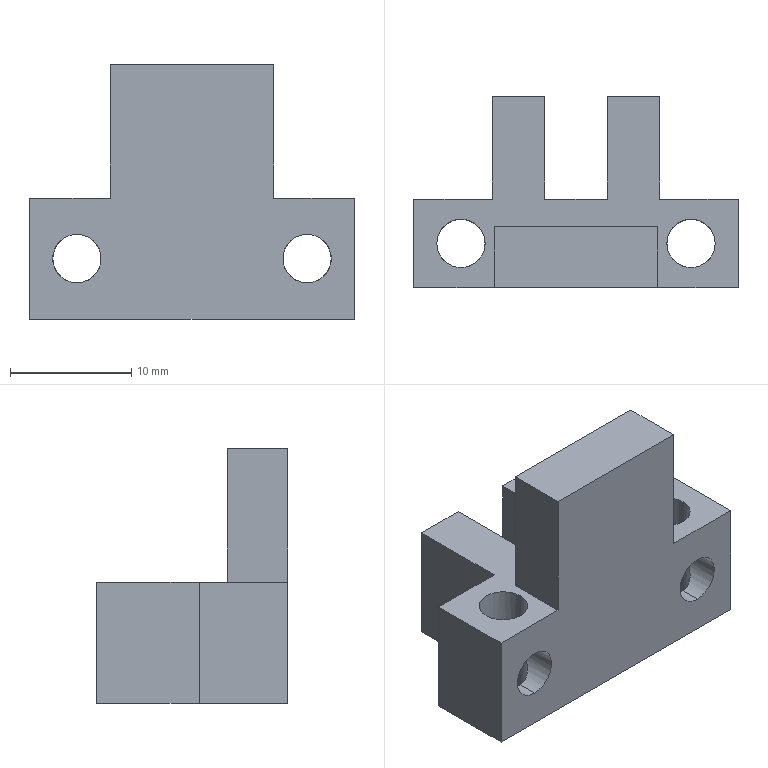Part | STEP file | PN_0024 EE-SX-671 photoelectric switch | 1 solid | 124 faces | box 26.8 x 15.8 x 21 mm | volume 3068 mm3 | plane 84 | spline 24 | cylinder 16 | commonest cylinder face diameters 4 x16